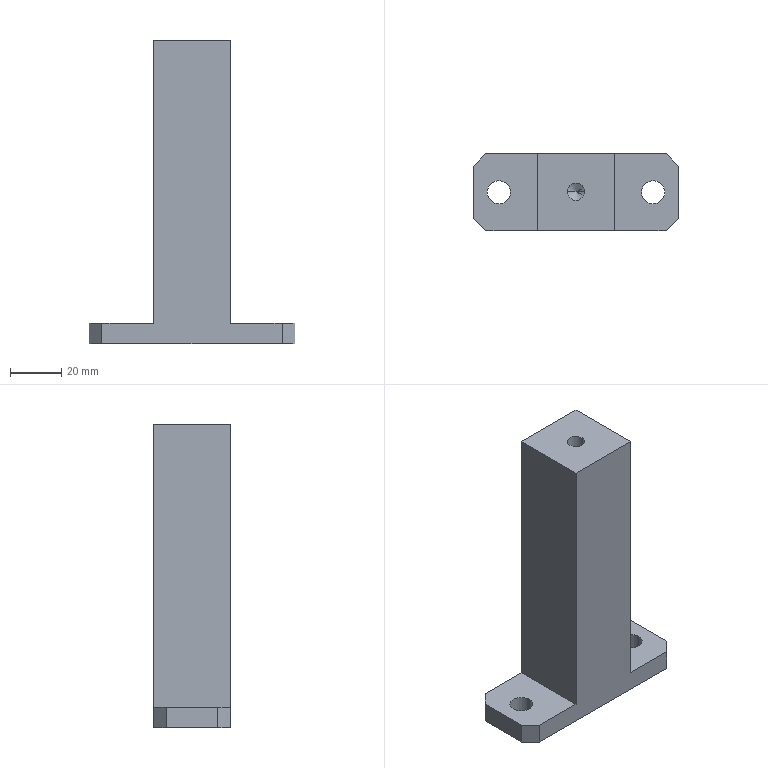Part | SolidWorks | features ICE 2, 3DProfileFeature 1, Extrusion 1, HoleWzd 1 | 1 solid | 22 faces | box 80 x 30 x 118 mm | volume 115849 mm3 | plane 14 | cylinder 6 | cone 2 | commonest cylinder face diameters 9 x4 6.8 x2
STEP:
#1=CARTESIAN_POINT('',(-3.4,0.,93.));
#2=VERTEX_POINT('',#1);
#3=CARTESIAN_POINT('',(3.4,0.,93.));
#4=VERTEX_POINT('',#3);
#5=CARTESIAN_POINT('',(0.,0.,93.));
#6=DIRECTION('',(0.,0.,1.));
#7=DIRECTION('',(1.,0.,0.));
#8=AXIS2_PLACEMENT_3D('',#5,#6,#7);
#9=CIRCLE('',#8,3.4);
#10=EDGE_CURVE('',#2,#4,#9,.T.);
#11=ORIENTED_EDGE('',*,*,#10,.F.);
#12=CARTESIAN_POINT('',(-3.4,0.,118.));
#13=VERTEX_POINT('',#12);
#14=CARTESIAN_POINT('',(-3.4,0.,118.));
#15=DIRECTION('',(0.,0.,1.));
#16=VECTOR('',#15,1000.);
#17=LINE('',#14,#16);
#18=EDGE_CURVE('',#2,#13,#17,.T.);
#19=ORIENTED_EDGE('',*,*,#18,.T.);
#20=CARTESIAN_POINT('',(3.4,0.,118.));
#21=VERTEX_POINT('',#20);
#22=CARTESIAN_POINT('',(0.,0.,118.));
#23=DIRECTION('',(0.,0.,1.));
#24=DIRECTION('',(1.,0.,0.));
#25=AXIS2_PLACEMENT_3D('',#22,#23,#24);
#26=CIRCLE('',#25,3.4);
#27=EDGE_CURVE('',#13,#21,#26,.T.);
#28=ORIENTED_EDGE('',*,*,#27,.T.);
#29=CARTESIAN_POINT('',(3.4,0.,118.));
#30=DIRECTION('',(0.,0.,1.));
#31=VECTOR('',#30,1000.);
#32=LINE('',#29,#31);
#33=EDGE_CURVE('',#4,#21,#32,.T.);
#34=ORIENTED_EDGE('',*,*,#33,.F.);
#35=EDGE_LOOP('',(#11,#19,#28,#34));
#36=FACE_OUTER_BOUND('',#35,.T.);
#37=CARTESIAN_POINT('',(0.,0.,118.));
#38=DIRECTION('',(0.,0.,1.));
#39=DIRECTION('',(1.,0.,0.));
#40=AXIS2_PLACEMENT_3D('',#37,#38,#39);
#41=CYLINDRICAL_SURFACE('',#40,3.4);
#42=ADVANCED_FACE('',(#36),#41,.F.);
#43=CARTESIAN_POINT('',(0.,0.,90.957));
#44=VERTEX_POINT('',#43);
#45=CARTESIAN_POINT('',(3.4,0.,93.));
#46=DIRECTION('',(0.8572,0.,0.515));
#47=VECTOR('',#46,1000.);
#48=LINE('',#45,#47);
#49=EDGE_CURVE('',#44,#4,#48,.T.);
#50=ORIENTED_EDGE('',*,*,#49,.F.);
#51=CARTESIAN_POINT('',(-3.4,0.,93.));
#52=DIRECTION('',(-0.8572,0.,0.515));
#53=VECTOR('',#52,1000.);
#54=LINE('',#51,#53);
#55=EDGE_CURVE('',#44,#2,#54,.T.);
#56=ORIENTED_EDGE('',*,*,#55,.T.);
#57=ORIENTED_EDGE('',*,*,#10,.T.);
#58=EDGE_LOOP('',(#50,#56,#57));
#59=FACE_OUTER_BOUND('',#58,.T.);
#60=CARTESIAN_POINT('',(0.,0.,93.));
#61=DIRECTION('',(0.,0.,1.));
#62=DIRECTION('',(1.,0.,0.));
#63=AXIS2_PLACEMENT_3D('',#60,#61,#62);
#64=CONICAL_SURFACE('',#63,3.4,1.03);
#65=ADVANCED_FACE('',(#59),#64,.F.);
#66=CARTESIAN_POINT('',(25.5,0.,8.));
#67=VERTEX_POINT('',#66);
#68=CARTESIAN_POINT('',(34.5,0.,8.));
#69=VERTEX_POINT('',#68);
#70=CARTESIAN_POINT('',(30.,0.,8.));
#71=DIRECTION('',(0.,0.,1.));
#72=DIRECTION('',(1.,0.,0.));
#73=AXIS2_PLACEMENT_3D('',#70,#71,#72);
#74=CIRCLE('',#73,4.5);
#75=EDGE_CURVE('',#67,#69,#74,.T.);
#76=ORIENTED_EDGE('',*,*,#75,.T.);
#77=CARTESIAN_POINT('',(34.5,0.,0.));
#78=VERTEX_POINT('',#77);
#79=CARTESIAN_POINT('',(34.5,0.,8.));
#80=DIRECTION('',(0.,0.,-1.));
#81=VECTOR('',#80,1000.);
#82=LINE('',#79,#81);
#83=EDGE_CURVE('',#69,#78,#82,.T.);
#84=ORIENTED_EDGE('',*,*,#83,.T.);
#85=CARTESIAN_POINT('',(25.5,0.,0.));
#86=VERTEX_POINT('',#85);
#87=CARTESIAN_POINT('',(30.,0.,0.));
#88=DIRECTION('',(0.,0.,1.));
#89=DIRECTION('',(1.,0.,0.));
#90=AXIS2_PLACEMENT_3D('',#87,#88,#89);
#91=CIRCLE('',#90,4.5);
#92=EDGE_CURVE('',#86,#78,#91,.T.);
#93=ORIENTED_EDGE('',*,*,#92,.F.);
#94=CARTESIAN_POINT('',(25.5,0.,8.));
#95=DIRECTION('',(0.,0.,-1.));
#96=VECTOR('',#95,1000.);
#97=LINE('',#94,#96);
#98=EDGE_CURVE('',#67,#86,#97,.T.);
#99=ORIENTED_EDGE('',*,*,#98,.F.);
#100=EDGE_LOOP('',(#76,#84,#93,#99));
#101=FACE_OUTER_BOUND('',#100,.T.);
#102=CARTESIAN_POINT('',(30.,0.,8.));
#103=DIRECTION('',(0.,0.,-1.));
#104=DIRECTION('',(-1.,0.,0.));
#105=AXIS2_PLACEMENT_3D('',#102,#103,#104);
#106=CYLINDRICAL_SURFACE('',#105,4.5);
#107=ADVANCED_FACE('',(#101),#106,.F.);
#108=CARTESIAN_POINT('',(-34.5,0.,8.));
#109=VERTEX_POINT('',#108);
#110=CARTESIAN_POINT('',(-25.5,0.,8.));
#111=VERTEX_POINT('',#110);
#112=CARTESIAN_POINT('',(-30.,0.,8.));
#113=DIRECTION('',(0.,0.,1.));
#114=DIRECTION('',(1.,0.,0.));
#115=AXIS2_PLACEMENT_3D('',#112,#113,#114);
#116=CIRCLE('',#115,4.5);
#117=EDGE_CURVE('',#109,#111,#116,.T.);
#118=ORIENTED_EDGE('',*,*,#117,.T.);
#119=CARTESIAN_POINT('',(-25.5,0.,0.));
#120=VERTEX_POINT('',#119);
#121=CARTESIAN_POINT('',(-25.5,0.,8.));
#122=DIRECTION('',(0.,0.,-1.));
#123=VECTOR('',#122,1000.);
#124=LINE('',#121,#123);
#125=EDGE_CURVE('',#111,#120,#124,.T.);
#126=ORIENTED_EDGE('',*,*,#125,.T.);
#127=CARTESIAN_POINT('',(-34.5,0.,0.));
#128=VERTEX_POINT('',#127);
#129=CARTESIAN_POINT('',(-30.,0.,0.));
#130=DIRECTION('',(0.,0.,1.));
#131=DIRECTION('',(1.,0.,0.));
#132=AXIS2_PLACEMENT_3D('',#129,#130,#131);
#133=CIRCLE('',#132,4.5);
#134=EDGE_CURVE('',#128,#120,#133,.T.);
#135=ORIENTED_EDGE('',*,*,#134,.F.);
#136=CARTESIAN_POINT('',(-34.5,0.,8.));
#137=DIRECTION('',(0.,0.,-1.));
#138=VECTOR('',#137,1000.);
#139=LINE('',#136,#138);
#140=EDGE_CURVE('',#109,#128,#139,.T.);
#141=ORIENTED_EDGE('',*,*,#140,.F.);
#142=EDGE_LOOP('',(#118,#126,#135,#141));
#143=FACE_OUTER_BOUND('',#142,.T.);
#144=CARTESIAN_POINT('',(-30.,0.,8.));
#145=DIRECTION('',(0.,0.,-1.));
#146=DIRECTION('',(-1.,0.,0.));
#147=AXIS2_PLACEMENT_3D('',#144,#145,#146);
#148=CYLINDRICAL_SURFACE('',#147,4.5);
#149=ADVANCED_FACE('',(#143),#148,.F.);
#150=CARTESIAN_POINT('',(-15.,15.,8.));
#151=VERTEX_POINT('',#150);
#152=CARTESIAN_POINT('',(-15.,-15.,8.));
#153=VERTEX_POINT('',#152);
#154=CARTESIAN_POINT('',(-15.,-15.,8.));
#155=DIRECTION('',(0.,-1.,0.));
#156=VECTOR('',#155,1000.);
#157=LINE('',#154,#156);
#158=EDGE_CURVE('',#151,#153,#157,.T.);
#159=ORIENTED_EDGE('',*,*,#158,.F.);
#160=CARTESIAN_POINT('',(-35.,15.,8.));
#161=VERTEX_POINT('',#160);
#162=CARTESIAN_POINT('',(35.,15.,8.));
#163=DIRECTION('',(-1.,0.,0.));
#164=VECTOR('',#163,1000.);
#165=LINE('',#162,#164);
#166=EDGE_CURVE('',#151,#161,#165,.T.);
#167=ORIENTED_EDGE('',*,*,#166,.T.);
#168=CARTESIAN_POINT('',(-40.,10.,8.));
#169=VERTEX_POINT('',#168);
#170=CARTESIAN_POINT('',(-40.,10.,8.));
#171=DIRECTION('',(-0.7071,-0.7071,0.));
#172=VECTOR('',#171,1000.);
#173=LINE('',#170,#172);
#174=EDGE_CURVE('',#161,#169,#173,.T.);
#175=ORIENTED_EDGE('',*,*,#174,.T.);
#176=CARTESIAN_POINT('',(-40.,-10.,8.));
#177=VERTEX_POINT('',#176);
#178=CARTESIAN_POINT('',(-40.,-10.,8.));
#179=DIRECTION('',(0.,-1.,0.));
#180=VECTOR('',#179,1000.);
#181=LINE('',#178,#180);
#182=EDGE_CURVE('',#169,#177,#181,.T.);
#183=ORIENTED_EDGE('',*,*,#182,.T.);
#184=CARTESIAN_POINT('',(-35.,-15.,8.));
#185=VERTEX_POINT('',#184);
#186=CARTESIAN_POINT('',(-35.,-15.,8.));
#187=DIRECTION('',(0.7071,-0.7071,0.));
#188=VECTOR('',#187,1000.);
#189=LINE('',#186,#188);
#190=EDGE_CURVE('',#177,#185,#189,.T.);
#191=ORIENTED_EDGE('',*,*,#190,.T.);
#192=CARTESIAN_POINT('',(35.,-15.,8.));
#193=DIRECTION('',(1.,0.,0.));
#194=VECTOR('',#193,1000.);
#195=LINE('',#192,#194);
#196=EDGE_CURVE('',#185,#153,#195,.T.);
#197=ORIENTED_EDGE('',*,*,#196,.T.);
#198=EDGE_LOOP('',(#159,#167,#175,#183,#191,#197));
#199=FACE_OUTER_BOUND('',#198,.T.);
#200=ORIENTED_EDGE('',*,*,#117,.F.);
#201=CARTESIAN_POINT('',(-30.,0.,8.));
#202=DIRECTION('',(0.,0.,1.));
#203=DIRECTION('',(1.,0.,0.));
#204=AXIS2_PLACEMENT_3D('',#201,#202,#203);
#205=CIRCLE('',#204,4.5);
#206=EDGE_CURVE('',#111,#109,#205,.T.);
#207=ORIENTED_EDGE('',*,*,#206,.F.);
#208=EDGE_LOOP('',(#200,#207));
#209=FACE_BOUND('',#208,.T.);
#210=CARTESIAN_POINT('',(0.,0.,8.));
#211=DIRECTION('',(0.,0.,1.));
#212=DIRECTION('',(1.,0.,0.));
#213=AXIS2_PLACEMENT_3D('',#210,#211,#212);
#214=PLANE('',#213);
#215=ADVANCED_FACE('',(#199,#209),#214,.T.);
#216=CARTESIAN_POINT('',(15.,-15.,8.));
#217=VERTEX_POINT('',#216);
#218=CARTESIAN_POINT('',(15.,15.,8.));
#219=VERTEX_POINT('',#218);
#220=CARTESIAN_POINT('',(15.,-15.,8.));
#221=DIRECTION('',(0.,1.,0.));
#222=VECTOR('',#221,1000.);
#223=LINE('',#220,#222);
#224=EDGE_CURVE('',#217,#219,#223,.T.);
#225=ORIENTED_EDGE('',*,*,#224,.F.);
#226=CARTESIAN_POINT('',(35.,-15.,8.));
#227=VERTEX_POINT('',#226);
#228=CARTESIAN_POINT('',(35.,-15.,8.));
#229=DIRECTION('',(1.,0.,0.));
#230=VECTOR('',#229,1000.);
#231=LINE('',#228,#230);
#232=EDGE_CURVE('',#217,#227,#231,.T.);
#233=ORIENTED_EDGE('',*,*,#232,.T.);
#234=CARTESIAN_POINT('',(40.,-10.,8.));
#235=VERTEX_POINT('',#234);
#236=CARTESIAN_POINT('',(35.,-15.,8.));
#237=DIRECTION('',(0.7071,0.7071,0.));
#238=VECTOR('',#237,1000.);
#239=LINE('',#236,#238);
#240=EDGE_CURVE('',#227,#235,#239,.T.);
#241=ORIENTED_EDGE('',*,*,#240,.T.);
#242=CARTESIAN_POINT('',(40.,10.,8.));
#243=VERTEX_POINT('',#242);
#244=CARTESIAN_POINT('',(40.,-10.,8.));
#245=DIRECTION('',(0.,1.,0.));
#246=VECTOR('',#245,1000.);
#247=LINE('',#244,#246);
#248=EDGE_CURVE('',#235,#243,#247,.T.);
#249=ORIENTED_EDGE('',*,*,#248,.T.);
#250=CARTESIAN_POINT('',(35.,15.,8.));
#251=VERTEX_POINT('',#250);
#252=CARTESIAN_POINT('',(40.,10.,8.));
#253=DIRECTION('',(-0.7071,0.7071,0.));
#254=VECTOR('',#253,1000.);
#255=LINE('',#252,#254);
#256=EDGE_CURVE('',#243,#251,#255,.T.);
#257=ORIENTED_EDGE('',*,*,#256,.T.);
#258=CARTESIAN_POINT('',(35.,15.,8.));
#259=DIRECTION('',(-1.,0.,0.));
#260=VECTOR('',#259,1000.);
#261=LINE('',#258,#260);
#262=EDGE_CURVE('',#251,#219,#261,.T.);
#263=ORIENTED_EDGE('',*,*,#262,.T.);
#264=EDGE_LOOP('',(#225,#233,#241,#249,#257,#263));
#265=FACE_OUTER_BOUND('',#264,.T.);
#266=ORIENTED_EDGE('',*,*,#75,.F.);
#267=CARTESIAN_POINT('',(30.,0.,8.));
#268=DIRECTION('',(0.,0.,1.));
#269=DIRECTION('',(1.,0.,0.));
#270=AXIS2_PLACEMENT_3D('',#267,#268,#269);
#271=CIRCLE('',#270,4.5);
#272=EDGE_CURVE('',#69,#67,#271,.T.);
#273=ORIENTED_EDGE('',*,*,#272,.F.);
#274=EDGE_LOOP('',(#266,#273));
#275=FACE_BOUND('',#274,.T.);
#276=CARTESIAN_POINT('',(0.,0.,8.));
#277=DIRECTION('',(0.,0.,1.));
#278=DIRECTION('',(1.,0.,0.));
#279=AXIS2_PLACEMENT_3D('',#276,#277,#278);
#280=PLANE('',#279);
#281=ADVANCED_FACE('',(#265,#275),#280,.T.);
#282=CARTESIAN_POINT('',(-40.,10.,0.));
#283=VERTEX_POINT('',#282);
#284=CARTESIAN_POINT('',(-40.,-10.,0.));
#285=VERTEX_POINT('',#284);
#286=CARTESIAN_POINT('',(-40.,-10.,0.));
#287=DIRECTION('',(0.,-1.,0.));
#288=VECTOR('',#287,1000.);
#289=LINE('',#286,#288);
#290=EDGE_CURVE('',#283,#285,#289,.T.);
#291=ORIENTED_EDGE('',*,*,#290,.F.);
#292=CARTESIAN_POINT('',(-35.,15.,0.));
#293=VERTEX_POINT('',#292);
#294=CARTESIAN_POINT('',(-40.,10.,0.));
#295=DIRECTION('',(-0.7071,-0.7071,0.));
#296=VECTOR('',#295,1000.);
#297=LINE('',#294,#296);
#298=EDGE_CURVE('',#293,#283,#297,.T.);
#299=ORIENTED_EDGE('',*,*,#298,.F.);
#300=CARTESIAN_POINT('',(35.,15.,0.));
#301=VERTEX_POINT('',#300);
#302=CARTESIAN_POINT('',(35.,15.,0.));
#303=DIRECTION('',(-1.,0.,0.));
#304=VECTOR('',#303,1000.);
#305=LINE('',#302,#304);
#306=EDGE_CURVE('',#301,#293,#305,.T.);
#307=ORIENTED_EDGE('',*,*,#306,.F.);
#308=CARTESIAN_POINT('',(40.,10.,0.));
#309=VERTEX_POINT('',#308);
#310=CARTESIAN_POINT('',(40.,10.,0.));
#311=DIRECTION('',(-0.7071,0.7071,0.));
#312=VECTOR('',#311,1000.);
#313=LINE('',#310,#312);
#314=EDGE_CURVE('',#309,#301,#313,.T.);
#315=ORIENTED_EDGE('',*,*,#314,.F.);
#316=CARTESIAN_POINT('',(40.,-10.,0.));
#317=VERTEX_POINT('',#316);
#318=CARTESIAN_POINT('',(40.,-10.,0.));
#319=DIRECTION('',(0.,1.,0.));
#320=VECTOR('',#319,1000.);
#321=LINE('',#318,#320);
#322=EDGE_CURVE('',#317,#309,#321,.T.);
#323=ORIENTED_EDGE('',*,*,#322,.F.);
#324=CARTESIAN_POINT('',(35.,-15.,0.));
#325=VERTEX_POINT('',#324);
#326=CARTESIAN_POINT('',(35.,-15.,0.));
#327=DIRECTION('',(0.7071,0.7071,0.));
#328=VECTOR('',#327,1000.);
#329=LINE('',#326,#328);
#330=EDGE_CURVE('',#325,#317,#329,.T.);
#331=ORIENTED_EDGE('',*,*,#330,.F.);
#332=CARTESIAN_POINT('',(-35.,-15.,0.));
#333=VERTEX_POINT('',#332);
#334=CARTESIAN_POINT('',(35.,-15.,0.));
#335=DIRECTION('',(1.,0.,0.));
#336=VECTOR('',#335,1000.);
#337=LINE('',#334,#336);
#338=EDGE_CURVE('',#333,#325,#337,.T.);
#339=ORIENTED_EDGE('',*,*,#338,.F.);
#340=CARTESIAN_POINT('',(-35.,-15.,0.));
#341=DIRECTION('',(0.7071,-0.7071,0.));
#342=VECTOR('',#341,1000.);
#343=LINE('',#340,#342);
#344=EDGE_CURVE('',#285,#333,#343,.T.);
#345=ORIENTED_EDGE('',*,*,#344,.F.);
#346=EDGE_LOOP('',(#291,#299,#307,#315,#323,#331,#339,#345));
#347=FACE_OUTER_BOUND('',#346,.T.);
#348=ORIENTED_EDGE('',*,*,#134,.T.);
#349=CARTESIAN_POINT('',(-30.,0.,0.));
#350=DIRECTION('',(0.,0.,1.));
#351=DIRECTION('',(1.,0.,0.));
#352=AXIS2_PLACEMENT_3D('',#349,#350,#351);
#353=CIRCLE('',#352,4.5);
#354=EDGE_CURVE('',#120,#128,#353,.T.);
#355=ORIENTED_EDGE('',*,*,#354,.T.);
#356=EDGE_LOOP('',(#348,#355));
#357=FACE_BOUND('',#356,.T.);
#358=ORIENTED_EDGE('',*,*,#92,.T.);
#359=CARTESIAN_POINT('',(30.,0.,0.));
#360=DIRECTION('',(0.,0.,1.));
#361=DIRECTION('',(1.,0.,0.));
#362=AXIS2_PLACEMENT_3D('',#359,#360,#361);
#363=CIRCLE('',#362,4.5);
#364=EDGE_CURVE('',#78,#86,#363,.T.);
#365=ORIENTED_EDGE('',*,*,#364,.T.);
#366=EDGE_LOOP('',(#358,#365));
#367=FACE_BOUND('',#366,.T.);
#368=CARTESIAN_POINT('',(0.,0.,0.));
#369=DIRECTION('',(0.,0.,1.));
#370=DIRECTION('',(1.,0.,0.));
#371=AXIS2_PLACEMENT_3D('',#368,#369,#370);
#372=PLANE('',#371);
#373=ADVANCED_FACE('',(#347,#357,#367),#372,.F.);
#374=ORIENTED_EDGE('',*,*,#290,.T.);
#375=CARTESIAN_POINT('',(-40.,-10.,8.));
#376=DIRECTION('',(0.,0.,-1.));
#377=VECTOR('',#376,1000.);
#378=LINE('',#375,#377);
#379=EDGE_CURVE('',#177,#285,#378,.T.);
#380=ORIENTED_EDGE('',*,*,#379,.F.);
#381=ORIENTED_EDGE('',*,*,#182,.F.);
#382=CARTESIAN_POINT('',(-40.,10.,8.));
#383=DIRECTION('',(0.,0.,-1.));
#384=VECTOR('',#383,1000.);
#385=LINE('',#382,#384);
#386=EDGE_CURVE('',#169,#283,#385,.T.);
#387=ORIENTED_EDGE('',*,*,#386,.T.);
#388=EDGE_LOOP('',(#374,#380,#381,#387));
#389=FACE_OUTER_BOUND('',#388,.T.);
#390=CARTESIAN_POINT('',(-40.,-10.,8.));
#391=DIRECTION('',(1.,0.,0.));
#392=DIRECTION('',(0.,1.,0.));
#393=AXIS2_PLACEMENT_3D('',#390,#391,#392);
#394=PLANE('',#393);
#395=ADVANCED_FACE('',(#389),#394,.F.);
#396=ORIENTED_EDGE('',*,*,#344,.T.);
#397=CARTESIAN_POINT('',(-35.,-15.,8.));
#398=DIRECTION('',(0.,0.,-1.));
#399=VECTOR('',#398,1000.);
#400=LINE('',#397,#399);
#401=EDGE_CURVE('',#185,#333,#400,.T.);
#402=ORIENTED_EDGE('',*,*,#401,.F.);
#403=ORIENTED_EDGE('',*,*,#190,.F.);
#404=ORIENTED_EDGE('',*,*,#379,.T.);
#405=EDGE_LOOP('',(#396,#402,#403,#404));
#406=FACE_OUTER_BOUND('',#405,.T.);
#407=CARTESIAN_POINT('',(-35.,-15.,8.));
#408=DIRECTION('',(0.7071,0.7071,0.));
#409=DIRECTION('',(-0.7071,0.7071,0.));
#410=AXIS2_PLACEMENT_3D('',#407,#408,#409);
#411=PLANE('',#410);
#412=ADVANCED_FACE('',(#406),#411,.F.);
#413=ORIENTED_EDGE('',*,*,#338,.T.);
#414=CARTESIAN_POINT('',(35.,-15.,8.));
#415=DIRECTION('',(0.,0.,-1.));
#416=VECTOR('',#415,1000.);
#417=LINE('',#414,#416);
#418=EDGE_CURVE('',#227,#325,#417,.T.);
#419=ORIENTED_EDGE('',*,*,#418,.F.);
#420=ORIENTED_EDGE('',*,*,#232,.F.);
#421=CARTESIAN_POINT('',(15.,-15.,118.));
#422=VERTEX_POINT('',#421);
#423=CARTESIAN_POINT('',(15.,-15.,118.));
#424=DIRECTION('',(0.,0.,-1.));
#425=VECTOR('',#424,1000.);
#426=LINE('',#423,#425);
#427=EDGE_CURVE('',#422,#217,#426,.T.);
#428=ORIENTED_EDGE('',*,*,#427,.F.);
#429=CARTESIAN_POINT('',(-15.,-15.,118.));
#430=VERTEX_POINT('',#429);
#431=CARTESIAN_POINT('',(15.,-15.,118.));
#432=DIRECTION('',(1.,0.,0.));
#433=VECTOR('',#432,1000.);
#434=LINE('',#431,#433);
#435=EDGE_CURVE('',#430,#422,#434,.T.);
#436=ORIENTED_EDGE('',*,*,#435,.F.);
#437=CARTESIAN_POINT('',(-15.,-15.,118.));
#438=DIRECTION('',(0.,0.,-1.));
#439=VECTOR('',#438,1000.);
#440=LINE('',#437,#439);
#441=EDGE_CURVE('',#430,#153,#440,.T.);
#442=ORIENTED_EDGE('',*,*,#441,.T.);
#443=ORIENTED_EDGE('',*,*,#196,.F.);
#444=ORIENTED_EDGE('',*,*,#401,.T.);
#445=EDGE_LOOP('',(#413,#419,#420,#428,#436,#442,#443,#444));
#446=FACE_OUTER_BOUND('',#445,.T.);
#447=CARTESIAN_POINT('',(35.,-15.,8.));
#448=DIRECTION('',(0.,1.,0.));
#449=DIRECTION('',(-1.,0.,0.));
#450=AXIS2_PLACEMENT_3D('',#447,#448,#449);
#451=PLANE('',#450);
#452=ADVANCED_FACE('',(#446),#451,.F.);
#453=ORIENTED_EDGE('',*,*,#330,.T.);
#454=CARTESIAN_POINT('',(40.,-10.,8.));
#455=DIRECTION('',(0.,0.,-1.));
#456=VECTOR('',#455,1000.);
#457=LINE('',#454,#456);
#458=EDGE_CURVE('',#235,#317,#457,.T.);
#459=ORIENTED_EDGE('',*,*,#458,.F.);
#460=ORIENTED_EDGE('',*,*,#240,.F.);
#461=ORIENTED_EDGE('',*,*,#418,.T.);
#462=EDGE_LOOP('',(#453,#459,#460,#461));
#463=FACE_OUTER_BOUND('',#462,.T.);
#464=CARTESIAN_POINT('',(35.,-15.,8.));
#465=DIRECTION('',(-0.7071,0.7071,0.));
#466=DIRECTION('',(-0.7071,-0.7071,0.));
#467=AXIS2_PLACEMENT_3D('',#464,#465,#466);
#468=PLANE('',#467);
#469=ADVANCED_FACE('',(#463),#468,.F.);
#470=ORIENTED_EDGE('',*,*,#322,.T.);
#471=CARTESIAN_POINT('',(40.,10.,8.));
#472=DIRECTION('',(0.,0.,-1.));
#473=VECTOR('',#472,1000.);
#474=LINE('',#471,#473);
#475=EDGE_CURVE('',#243,#309,#474,.T.);
#476=ORIENTED_EDGE('',*,*,#475,.F.);
#477=ORIENTED_EDGE('',*,*,#248,.F.);
#478=ORIENTED_EDGE('',*,*,#458,.T.);
#479=EDGE_LOOP('',(#470,#476,#477,#478));
#480=FACE_OUTER_BOUND('',#479,.T.);
#481=CARTESIAN_POINT('',(40.,-10.,8.));
#482=DIRECTION('',(-1.,0.,0.));
#483=DIRECTION('',(0.,0.,1.));
#484=AXIS2_PLACEMENT_3D('',#481,#482,#483);
#485=PLANE('',#484);
#486=ADVANCED_FACE('',(#480),#485,.F.);
#487=ORIENTED_EDGE('',*,*,#314,.T.);
#488=CARTESIAN_POINT('',(35.,15.,8.));
#489=DIRECTION('',(0.,0.,-1.));
#490=VECTOR('',#489,1000.);
#491=LINE('',#488,#490);
#492=EDGE_CURVE('',#251,#301,#491,.T.);
#493=ORIENTED_EDGE('',*,*,#492,.F.);
#494=ORIENTED_EDGE('',*,*,#256,.F.);
#495=ORIENTED_EDGE('',*,*,#475,.T.);
#496=EDGE_LOOP('',(#487,#493,#494,#495));
#497=FACE_OUTER_BOUND('',#496,.T.);
#498=CARTESIAN_POINT('',(40.,10.,8.));
#499=DIRECTION('',(-0.7071,-0.7071,0.));
#500=DIRECTION('',(0.7071,-0.7071,0.));
#501=AXIS2_PLACEMENT_3D('',#498,#499,#500);
#502=PLANE('',#501);
#503=ADVANCED_FACE('',(#497),#502,.F.);
#504=ORIENTED_EDGE('',*,*,#306,.T.);
#505=CARTESIAN_POINT('',(-35.,15.,8.));
#506=DIRECTION('',(0.,0.,-1.));
#507=VECTOR('',#506,1000.);
#508=LINE('',#505,#507);
#509=EDGE_CURVE('',#161,#293,#508,.T.);
#510=ORIENTED_EDGE('',*,*,#509,.F.);
#511=ORIENTED_EDGE('',*,*,#166,.F.);
#512=CARTESIAN_POINT('',(-15.,15.,118.));
#513=VERTEX_POINT('',#512);
#514=CARTESIAN_POINT('',(-15.,15.,118.));
#515=DIRECTION('',(0.,0.,-1.));
#516=VECTOR('',#515,1000.);
#517=LINE('',#514,#516);
#518=EDGE_CURVE('',#513,#151,#517,.T.);
#519=ORIENTED_EDGE('',*,*,#518,.F.);
#520=CARTESIAN_POINT('',(15.,15.,118.));
#521=VERTEX_POINT('',#520);
#522=CARTESIAN_POINT('',(15.,15.,118.));
#523=DIRECTION('',(-1.,0.,0.));
#524=VECTOR('',#523,1000.);
#525=LINE('',#522,#524);
#526=EDGE_CURVE('',#521,#513,#525,.T.);
#527=ORIENTED_EDGE('',*,*,#526,.F.);
#528=CARTESIAN_POINT('',(15.,15.,118.));
#529=DIRECTION('',(0.,0.,-1.));
#530=VECTOR('',#529,1000.);
#531=LINE('',#528,#530);
#532=EDGE_CURVE('',#521,#219,#531,.T.);
#533=ORIENTED_EDGE('',*,*,#532,.T.);
#534=ORIENTED_EDGE('',*,*,#262,.F.);
#535=ORIENTED_EDGE('',*,*,#492,.T.);
#536=EDGE_LOOP('',(#504,#510,#511,#519,#527,#533,#534,#535));
#537=FACE_OUTER_BOUND('',#536,.T.);
#538=CARTESIAN_POINT('',(35.,15.,8.));
#539=DIRECTION('',(0.,-1.,0.));
#540=DIRECTION('',(1.,0.,0.));
#541=AXIS2_PLACEMENT_3D('',#538,#539,#540);
#542=PLANE('',#541);
#543=ADVANCED_FACE('',(#537),#542,.F.);
#544=ORIENTED_EDGE('',*,*,#298,.T.);
#545=ORIENTED_EDGE('',*,*,#386,.F.);
#546=ORIENTED_EDGE('',*,*,#174,.F.);
#547=ORIENTED_EDGE('',*,*,#509,.T.);
#548=EDGE_LOOP('',(#544,#545,#546,#547));
#549=FACE_OUTER_BOUND('',#548,.T.);
#550=CARTESIAN_POINT('',(-40.,10.,8.));
#551=DIRECTION('',(0.7071,-0.7071,0.));
#552=DIRECTION('',(0.7071,0.7071,0.));
#553=AXIS2_PLACEMENT_3D('',#550,#551,#552);
#554=PLANE('',#553);
#555=ADVANCED_FACE('',(#549),#554,.F.);
#556=ORIENTED_EDGE('',*,*,#125,.F.);
#557=ORIENTED_EDGE('',*,*,#206,.T.);
#558=ORIENTED_EDGE('',*,*,#140,.T.);
#559=ORIENTED_EDGE('',*,*,#354,.F.);
#560=EDGE_LOOP('',(#556,#557,#558,#559));
#561=FACE_OUTER_BOUND('',#560,.T.);
#562=CARTESIAN_POINT('',(-30.,0.,8.));
#563=DIRECTION('',(0.,0.,-1.));
#564=DIRECTION('',(-1.,0.,0.));
#565=AXIS2_PLACEMENT_3D('',#562,#563,#564);
#566=CYLINDRICAL_SURFACE('',#565,4.5);
#567=ADVANCED_FACE('',(#561),#566,.F.);
#568=ORIENTED_EDGE('',*,*,#83,.F.);
#569=ORIENTED_EDGE('',*,*,#272,.T.);
#570=ORIENTED_EDGE('',*,*,#98,.T.);
#571=ORIENTED_EDGE('',*,*,#364,.F.);
#572=EDGE_LOOP('',(#568,#569,#570,#571));
#573=FACE_OUTER_BOUND('',#572,.T.);
#574=CARTESIAN_POINT('',(30.,0.,8.));
#575=DIRECTION('',(0.,0.,-1.));
#576=DIRECTION('',(-1.,0.,0.));
#577=AXIS2_PLACEMENT_3D('',#574,#575,#576);
#578=CYLINDRICAL_SURFACE('',#577,4.5);
#579=ADVANCED_FACE('',(#573),#578,.F.);
#580=ORIENTED_EDGE('',*,*,#158,.T.);
#581=ORIENTED_EDGE('',*,*,#441,.F.);
#582=CARTESIAN_POINT('',(-15.,-15.,118.));
#583=DIRECTION('',(0.,-1.,0.));
#584=VECTOR('',#583,1000.);
#585=LINE('',#582,#584);
#586=EDGE_CURVE('',#513,#430,#585,.T.);
#587=ORIENTED_EDGE('',*,*,#586,.F.);
#588=ORIENTED_EDGE('',*,*,#518,.T.);
#589=EDGE_LOOP('',(#580,#581,#587,#588));
#590=FACE_OUTER_BOUND('',#589,.T.);
#591=CARTESIAN_POINT('',(-15.,-15.,118.));
#592=DIRECTION('',(1.,0.,0.));
#593=DIRECTION('',(0.,0.,-1.));
#594=AXIS2_PLACEMENT_3D('',#591,#592,#593);
#595=PLANE('',#594);
#596=ADVANCED_FACE('',(#590),#595,.F.);
#597=ORIENTED_EDGE('',*,*,#224,.T.);
#598=ORIENTED_EDGE('',*,*,#532,.F.);
#599=CARTESIAN_POINT('',(15.,-15.,118.));
#600=DIRECTION('',(0.,1.,0.));
#601=VECTOR('',#600,1000.);
#602=LINE('',#599,#601);
#603=EDGE_CURVE('',#422,#521,#602,.T.);
#604=ORIENTED_EDGE('',*,*,#603,.F.);
#605=ORIENTED_EDGE('',*,*,#427,.T.);
#606=EDGE_LOOP('',(#597,#598,#604,#605));
#607=FACE_OUTER_BOUND('',#606,.T.);
#608=CARTESIAN_POINT('',(15.,-15.,118.));
#609=DIRECTION('',(-1.,0.,0.));
#610=DIRECTION('',(0.,0.,1.));
#611=AXIS2_PLACEMENT_3D('',#608,#609,#610);
#612=PLANE('',#611);
#613=ADVANCED_FACE('',(#607),#612,.F.);
#614=CARTESIAN_POINT('',(0.,0.,118.));
#615=DIRECTION('',(0.,0.,1.));
#616=DIRECTION('',(1.,0.,0.));
#617=AXIS2_PLACEMENT_3D('',#614,#615,#616);
#618=CIRCLE('',#617,3.4);
#619=EDGE_CURVE('',#21,#13,#618,.T.);
#620=ORIENTED_EDGE('',*,*,#619,.F.);
#621=ORIENTED_EDGE('',*,*,#27,.F.);
#622=EDGE_LOOP('',(#620,#621));
#623=FACE_BOUND('',#622,.T.);
#624=ORIENTED_EDGE('',*,*,#586,.T.);
#625=ORIENTED_EDGE('',*,*,#435,.T.);
#626=ORIENTED_EDGE('',*,*,#603,.T.);
#627=ORIENTED_EDGE('',*,*,#526,.T.);
#628=EDGE_LOOP('',(#624,#625,#626,#627));
#629=FACE_OUTER_BOUND('',#628,.T.);
#630=CARTESIAN_POINT('',(0.,0.,118.));
#631=DIRECTION('',(0.,0.,1.));
#632=DIRECTION('',(1.,0.,0.));
#633=AXIS2_PLACEMENT_3D('',#630,#631,#632);
#634=PLANE('',#633);
#635=ADVANCED_FACE('',(#623,#629),#634,.T.);
#636=ORIENTED_EDGE('',*,*,#55,.F.);
#637=ORIENTED_EDGE('',*,*,#49,.T.);
#638=CARTESIAN_POINT('',(0.,0.,93.));
#639=DIRECTION('',(0.,0.,1.));
#640=DIRECTION('',(1.,0.,0.));
#641=AXIS2_PLACEMENT_3D('',#638,#639,#640);
#642=CIRCLE('',#641,3.4);
#643=EDGE_CURVE('',#4,#2,#642,.T.);
#644=ORIENTED_EDGE('',*,*,#643,.T.);
#645=EDGE_LOOP('',(#636,#637,#644));
#646=FACE_OUTER_BOUND('',#645,.T.);
#647=CARTESIAN_POINT('',(0.,0.,93.));
#648=DIRECTION('',(0.,0.,1.));
#649=DIRECTION('',(1.,0.,0.));
#650=AXIS2_PLACEMENT_3D('',#647,#648,#649);
#651=CONICAL_SURFACE('',#650,3.4,1.03);
#652=ADVANCED_FACE('',(#646),#651,.F.);
#653=ORIENTED_EDGE('',*,*,#18,.F.);
#654=ORIENTED_EDGE('',*,*,#643,.F.);
#655=ORIENTED_EDGE('',*,*,#33,.T.);
#656=ORIENTED_EDGE('',*,*,#619,.T.);
#657=EDGE_LOOP('',(#653,#654,#655,#656));
#658=FACE_OUTER_BOUND('',#657,.T.);
#659=CARTESIAN_POINT('',(0.,0.,118.));
#660=DIRECTION('',(0.,0.,1.));
#661=DIRECTION('',(1.,0.,0.));
#662=AXIS2_PLACEMENT_3D('',#659,#660,#661);
#663=CYLINDRICAL_SURFACE('',#662,3.4);
#664=ADVANCED_FACE('',(#658),#663,.F.);
#665=CLOSED_SHELL('',(#42,#65,#107,#149,#215,#281,#373,#395,#412,#452,#469,#486,#503,#543,#555,#567,#579,#596,#613,#635,#652,#664));
#666=MANIFOLD_SOLID_BREP('',#665);
#667=CARTESIAN_POINT('',(0.,0.,0.));
#668=DIRECTION('',(0.,0.,1.));
#669=DIRECTION('',(1.,0.,0.));
#670=AXIS2_PLACEMENT_3D('',#667,#668,#669);
#671=(LENGTH_UNIT()NAMED_UNIT(*)SI_UNIT(.MILLI.,.METRE.));
#672=UNCERTAINTY_MEASURE_WITH_UNIT(LENGTH_MEASURE(0.00001),#671,'','');
#673=(NAMED_UNIT(*)PLANE_ANGLE_UNIT()SI_UNIT($,.RADIAN.));
#674=(NAMED_UNIT(*)SI_UNIT($,.STERADIAN.)SOLID_ANGLE_UNIT());
#675=(GEOMETRIC_REPRESENTATION_CONTEXT(3)GLOBAL_UNCERTAINTY_ASSIGNED_CONTEXT((#672))GLOBAL_UNIT_ASSIGNED_CONTEXT((#671,#673,#674))REPRESENTATION_CONTEXT('',''));
#676=ADVANCED_BREP_SHAPE_REPRESENTATION('',(#666,#670),#675);